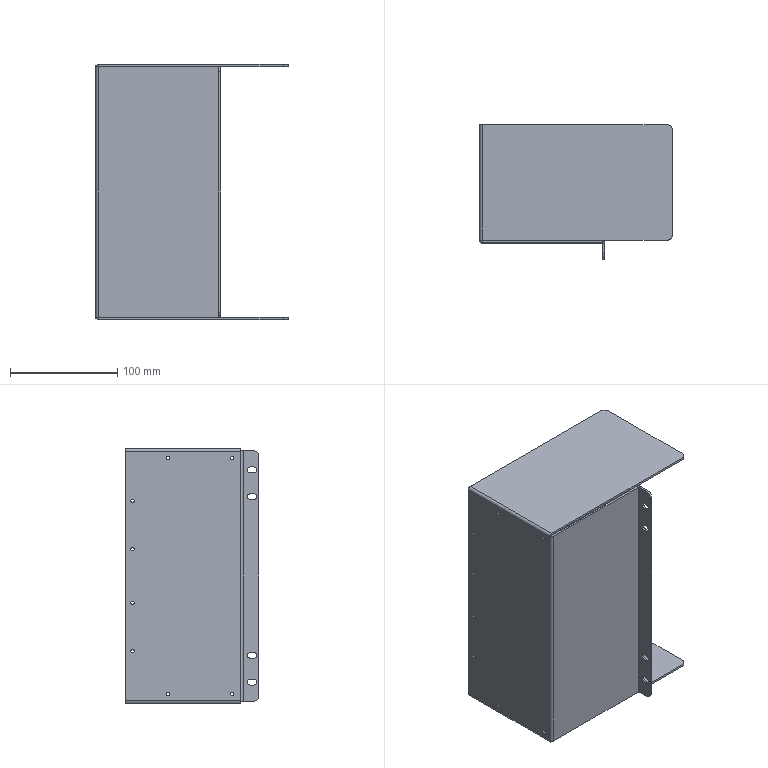Part | STEP file | 1 solid | 78 faces | box 180 x 125 x 238 mm | volume 188317 mm3 | plane 40 | cylinder 38 | commonest cylinder face diameters 3.3 x16 5.5 x8 10 x6 1 x4 5 x4